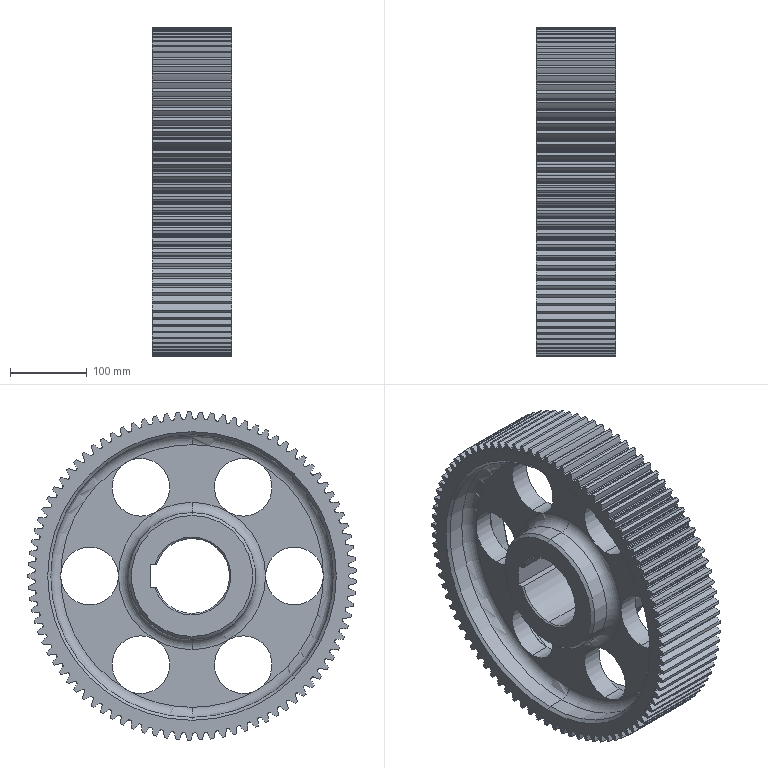Part | SolidWorks | features ICE 6, Chamfer 5, Revolution 1, Scale 1 | 1 solid | 638 faces | box 103.125 x 426.489 x 426.547 mm | volume 6214013 mm3 | cylinder 597 | plane 19 | cone 14 | torus 8 | commonest cylinder face diameters 3.75 x214 143.1 x182 426.563 x89 407.812 x88 75 x12 165 x4